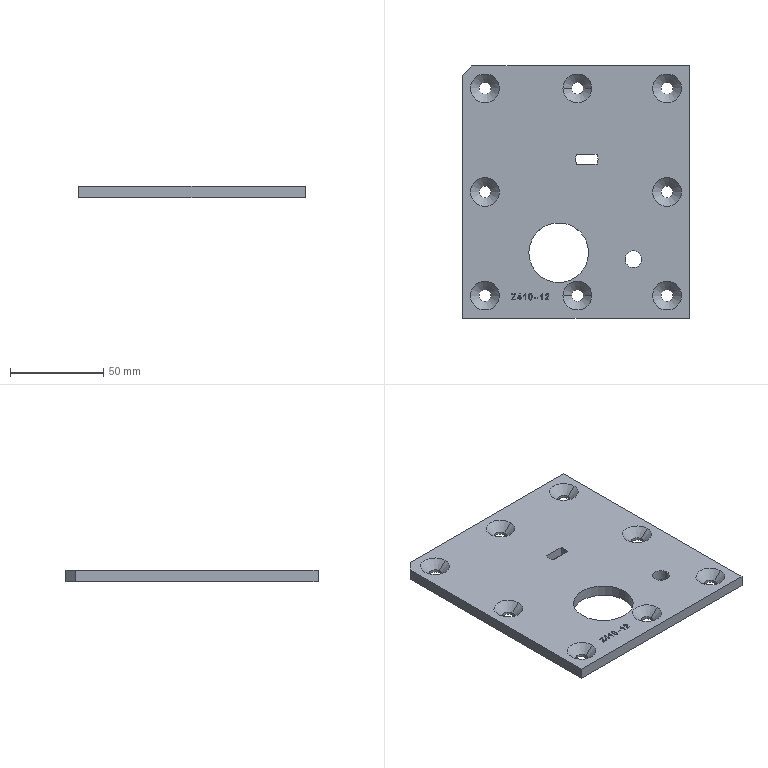Part | Creo | 1 solid | 148 faces | box 121.5 x 135 x 6 mm | volume 88789 mm3 | plane 57 | other 51 | cylinder 24 | cone 16 | commonest cylinder face diameters 6.4 x16 9 x2 12.2 x2 32 x2 2.89 x1 45.582 x1